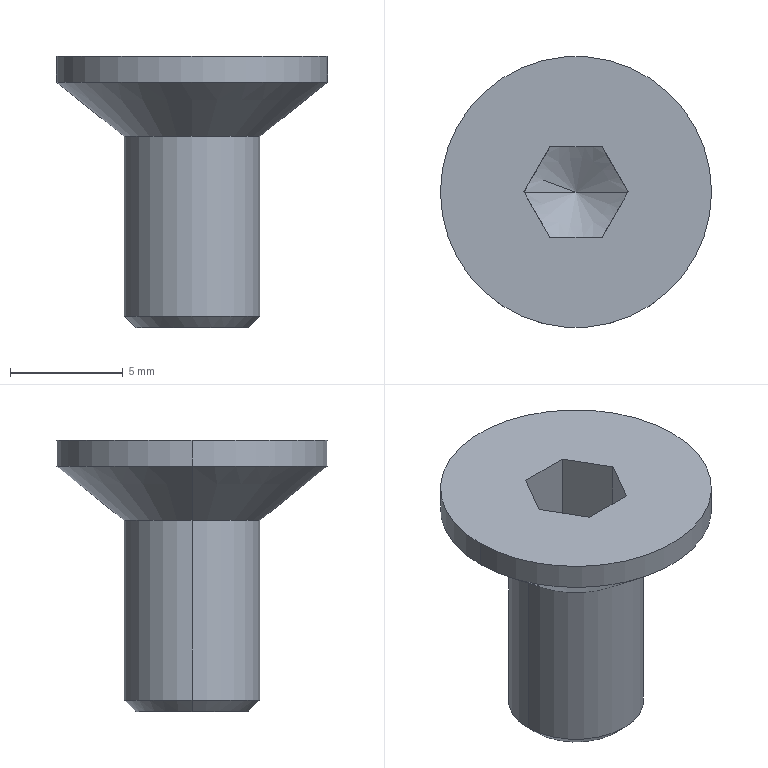Part | Creo | 1 solid | 18 faces | box 12 x 12 x 12 mm | volume 475.431 mm3 | plane 8 | cone 6 | cylinder 4 | commonest cylinder face diameters 6 x2 12 x2
STEP:
#1=CARTESIAN_POINT('',(219.809,61.745,-57.491));
#2=VERTEX_POINT('',#1);
#3=CARTESIAN_POINT('',(218.655,63.745,-57.491));
#4=VERTEX_POINT('',#3);
#5=CARTESIAN_POINT('',(219.809,61.745,-57.491));
#6=CARTESIAN_POINT('',(219.756,61.838,-57.522));
#7=CARTESIAN_POINT('',(219.648,62.026,-57.578));
#8=CARTESIAN_POINT('',(219.482,62.312,-57.639));
#9=CARTESIAN_POINT('',(219.315,62.601,-57.671));
#10=CARTESIAN_POINT('',(219.148,62.891,-57.671));
#11=CARTESIAN_POINT('',(218.981,63.18,-57.639));
#12=CARTESIAN_POINT('',(218.816,63.466,-57.578));
#13=CARTESIAN_POINT('',(218.708,63.653,-57.522));
#14=CARTESIAN_POINT('',(218.655,63.745,-57.491));
#15=B_SPLINE_CURVE_WITH_KNOTS('',3,(#5,#6,#7,#8,#9,#10,#11,#12,#13,#14),.UNSPECIFIED.,.F.,.F.,(4,1,1,1,1,1,1,4),(0.,0.1429,0.2857,0.4286,0.5714,0.7143,0.8571,1.),.UNSPECIFIED.);
#16=EDGE_CURVE('',#2,#4,#15,.T.);
#17=ORIENTED_EDGE('',*,*,#16,.F.);
#18=CARTESIAN_POINT('',(217.5,61.745,-58.824));
#19=VERTEX_POINT('',#18);
#20=CARTESIAN_POINT('',(217.5,61.745,-58.824));
#21=DIRECTION('',(0.866,0.,0.5));
#22=VECTOR('',#21,2.667);
#23=LINE('',#20,#22);
#24=EDGE_CURVE('',#19,#2,#23,.T.);
#25=ORIENTED_EDGE('',*,*,#24,.F.);
#26=CARTESIAN_POINT('',(215.191,61.745,-57.491));
#27=VERTEX_POINT('',#26);
#28=CARTESIAN_POINT('',(217.5,61.745,-58.824));
#29=DIRECTION('',(-0.866,0.,0.5));
#30=VECTOR('',#29,2.667);
#31=LINE('',#28,#30);
#32=EDGE_CURVE('',#19,#27,#31,.T.);
#33=ORIENTED_EDGE('',*,*,#32,.T.);
#34=CARTESIAN_POINT('',(216.345,63.745,-57.491));
#35=VERTEX_POINT('',#34);
#36=CARTESIAN_POINT('',(216.345,63.745,-57.491));
#37=CARTESIAN_POINT('',(216.292,63.653,-57.522));
#38=CARTESIAN_POINT('',(216.184,63.466,-57.578));
#39=CARTESIAN_POINT('',(216.019,63.18,-57.639));
#40=CARTESIAN_POINT('',(215.852,62.891,-57.671));
#41=CARTESIAN_POINT('',(215.685,62.601,-57.671));
#42=CARTESIAN_POINT('',(215.518,62.312,-57.639));
#43=CARTESIAN_POINT('',(215.352,62.026,-57.578));
#44=CARTESIAN_POINT('',(215.244,61.838,-57.522));
#45=CARTESIAN_POINT('',(215.191,61.745,-57.491));
#46=B_SPLINE_CURVE_WITH_KNOTS('',3,(#36,#37,#38,#39,#40,#41,#42,#43,#44,#45),.UNSPECIFIED.,.F.,.F.,(4,1,1,1,1,1,1,4),(0.,0.1429,0.2857,0.4286,0.5714,0.7143,0.8571,1.),.UNSPECIFIED.);
#47=EDGE_CURVE('',#35,#27,#46,.T.);
#48=ORIENTED_EDGE('',*,*,#47,.F.);
#49=CARTESIAN_POINT('',(218.655,63.745,-57.491));
#50=CARTESIAN_POINT('',(218.597,63.745,-57.508));
#51=CARTESIAN_POINT('',(218.483,63.745,-57.539));
#52=CARTESIAN_POINT('',(218.318,63.745,-57.578));
#53=CARTESIAN_POINT('',(218.156,63.745,-57.61));
#54=CARTESIAN_POINT('',(217.994,63.745,-57.636));
#55=CARTESIAN_POINT('',(217.831,63.745,-57.655));
#56=CARTESIAN_POINT('',(217.666,63.745,-57.667));
#57=CARTESIAN_POINT('',(217.5,63.745,-57.671));
#58=CARTESIAN_POINT('',(217.334,63.745,-57.667));
#59=CARTESIAN_POINT('',(217.169,63.745,-57.655));
#60=CARTESIAN_POINT('',(217.006,63.745,-57.636));
#61=CARTESIAN_POINT('',(216.844,63.745,-57.61));
#62=CARTESIAN_POINT('',(216.682,63.745,-57.578));
#63=CARTESIAN_POINT('',(216.517,63.745,-57.539));
#64=CARTESIAN_POINT('',(216.403,63.745,-57.508));
#65=CARTESIAN_POINT('',(216.345,63.745,-57.491));
#66=B_SPLINE_CURVE_WITH_KNOTS('',3,(#49,#50,#51,#52,#53,#54,#55,#56,#57,#58,#59,#60,#61,#62,#63,#64,#65),.UNSPECIFIED.,.F.,.F.,(4,1,1,1,1,1,1,1,1,1,1,1,1,1,4),(0.,0.07143,0.1429,0.2143,0.2857,0.3571,0.4286,0.5,0.5714,0.6429,0.7143,0.7857,0.8571,0.9286,1.),.UNSPECIFIED.);
#67=EDGE_CURVE('',#4,#35,#66,.T.);
#68=ORIENTED_EDGE('',*,*,#67,.F.);
#69=EDGE_LOOP('',(#17,#25,#33,#48,#68));
#70=FACE_OUTER_BOUND('',#69,.F.);
#71=CARTESIAN_POINT('',(217.5,61.745,-58.144));
#72=DIRECTION('',(0.,0.,1.));
#73=DIRECTION('',(1.,0.,0.));
#74=AXIS2_PLACEMENT_3D('',#71,#72,#73);
#75=CONICAL_SURFACE('',#74,1.178,60.);
#76=ADVANCED_FACE('',(#70),#75,.F.);
#77=CARTESIAN_POINT('',(218.655,63.745,-54.491));
#78=VERTEX_POINT('',#77);
#79=CARTESIAN_POINT('',(219.809,61.745,-54.491));
#80=VERTEX_POINT('',#79);
#81=CARTESIAN_POINT('',(218.655,63.745,-54.491));
#82=DIRECTION('',(0.5,-0.866,0.));
#83=VECTOR('',#82,2.309);
#84=LINE('',#81,#83);
#85=EDGE_CURVE('',#78,#80,#84,.T.);
#86=ORIENTED_EDGE('',*,*,#85,.T.);
#87=CARTESIAN_POINT('',(219.809,61.745,-54.491));
#88=DIRECTION('',(0.,0.,-1.));
#89=VECTOR('',#88,3.);
#90=LINE('',#87,#89);
#91=EDGE_CURVE('',#80,#2,#90,.T.);
#92=ORIENTED_EDGE('',*,*,#91,.T.);
#93=ORIENTED_EDGE('',*,*,#16,.T.);
#94=CARTESIAN_POINT('',(218.655,63.745,-54.491));
#95=DIRECTION('',(0.,0.,-1.));
#96=VECTOR('',#95,3.);
#97=LINE('',#94,#96);
#98=EDGE_CURVE('',#78,#4,#97,.T.);
#99=ORIENTED_EDGE('',*,*,#98,.F.);
#100=EDGE_LOOP('',(#86,#92,#93,#99));
#101=FACE_OUTER_BOUND('',#100,.F.);
#102=CARTESIAN_POINT('',(219.809,61.745,-57.491));
#103=DIRECTION('',(0.866,0.5,0.));
#104=DIRECTION('',(-0.5,0.866,0.));
#105=AXIS2_PLACEMENT_3D('',#102,#103,#104);
#106=PLANE('',#105);
#107=ADVANCED_FACE('',(#101),#106,.F.);
#108=CARTESIAN_POINT('',(223.5,61.745,-54.491));
#109=VERTEX_POINT('',#108);
#110=CARTESIAN_POINT('',(211.5,61.745,-54.491));
#111=VERTEX_POINT('',#110);
#112=CARTESIAN_POINT('',(217.5,61.745,-54.491));
#113=DIRECTION('',(0.,0.,1.));
#114=DIRECTION('',(1.,0.,0.));
#115=AXIS2_PLACEMENT_3D('',#112,#113,#114);
#116=CIRCLE('',#115,6.);
#117=EDGE_CURVE('',#109,#111,#116,.T.);
#118=ORIENTED_EDGE('',*,*,#117,.F.);
#119=CARTESIAN_POINT('',(217.5,61.745,-54.491));
#120=DIRECTION('',(0.,0.,1.));
#121=DIRECTION('',(-1.,0.,0.));
#122=AXIS2_PLACEMENT_3D('',#119,#120,#121);
#123=CIRCLE('',#122,6.);
#124=EDGE_CURVE('',#111,#109,#123,.T.);
#125=ORIENTED_EDGE('',*,*,#124,.F.);
#126=EDGE_LOOP('',(#118,#125));
#127=FACE_OUTER_BOUND('',#126,.F.);
#128=CARTESIAN_POINT('',(216.345,63.745,-54.491));
#129=VERTEX_POINT('',#128);
#130=CARTESIAN_POINT('',(216.345,63.745,-54.491));
#131=DIRECTION('',(1.,0.,0.));
#132=VECTOR('',#131,2.309);
#133=LINE('',#130,#132);
#134=EDGE_CURVE('',#129,#78,#133,.T.);
#135=ORIENTED_EDGE('',*,*,#134,.F.);
#136=CARTESIAN_POINT('',(215.191,61.745,-54.491));
#137=VERTEX_POINT('',#136);
#138=CARTESIAN_POINT('',(215.191,61.745,-54.491));
#139=DIRECTION('',(0.5,0.866,0.));
#140=VECTOR('',#139,2.309);
#141=LINE('',#138,#140);
#142=EDGE_CURVE('',#137,#129,#141,.T.);
#143=ORIENTED_EDGE('',*,*,#142,.F.);
#144=CARTESIAN_POINT('',(216.345,59.745,-54.491));
#145=VERTEX_POINT('',#144);
#146=CARTESIAN_POINT('',(216.345,59.745,-54.491));
#147=DIRECTION('',(-0.5,0.866,0.));
#148=VECTOR('',#147,2.309);
#149=LINE('',#146,#148);
#150=EDGE_CURVE('',#145,#137,#149,.T.);
#151=ORIENTED_EDGE('',*,*,#150,.F.);
#152=CARTESIAN_POINT('',(218.655,59.745,-54.491));
#153=VERTEX_POINT('',#152);
#154=CARTESIAN_POINT('',(218.655,59.745,-54.491));
#155=DIRECTION('',(-1.,0.,0.));
#156=VECTOR('',#155,2.309);
#157=LINE('',#154,#156);
#158=EDGE_CURVE('',#153,#145,#157,.T.);
#159=ORIENTED_EDGE('',*,*,#158,.F.);
#160=CARTESIAN_POINT('',(219.809,61.745,-54.491));
#161=DIRECTION('',(-0.5,-0.866,0.));
#162=VECTOR('',#161,2.309);
#163=LINE('',#160,#162);
#164=EDGE_CURVE('',#80,#153,#163,.T.);
#165=ORIENTED_EDGE('',*,*,#164,.F.);
#166=ORIENTED_EDGE('',*,*,#85,.F.);
#167=EDGE_LOOP('',(#135,#143,#151,#159,#165,#166));
#168=FACE_BOUND('',#167,.F.);
#169=CARTESIAN_POINT('',(223.5,61.745,-54.491));
#170=DIRECTION('',(0.,0.,-1.));
#171=DIRECTION('',(-1.,0.,0.));
#172=AXIS2_PLACEMENT_3D('',#169,#170,#171);
#173=PLANE('',#172);
#174=ADVANCED_FACE('',(#127,#168),#173,.F.);
#175=ORIENTED_EDGE('',*,*,#134,.T.);
#176=ORIENTED_EDGE('',*,*,#98,.T.);
#177=ORIENTED_EDGE('',*,*,#67,.T.);
#178=CARTESIAN_POINT('',(216.345,63.745,-54.491));
#179=DIRECTION('',(0.,0.,-1.));
#180=VECTOR('',#179,3.);
#181=LINE('',#178,#180);
#182=EDGE_CURVE('',#129,#35,#181,.T.);
#183=ORIENTED_EDGE('',*,*,#182,.F.);
#184=EDGE_LOOP('',(#175,#176,#177,#183));
#185=FACE_OUTER_BOUND('',#184,.F.);
#186=CARTESIAN_POINT('',(218.655,63.745,-57.491));
#187=DIRECTION('',(0.,1.,0.));
#188=DIRECTION('',(0.,0.,1.));
#189=AXIS2_PLACEMENT_3D('',#186,#187,#188);
#190=PLANE('',#189);
#191=ADVANCED_FACE('',(#185),#190,.F.);
#192=ORIENTED_EDGE('',*,*,#142,.T.);
#193=ORIENTED_EDGE('',*,*,#182,.T.);
#194=ORIENTED_EDGE('',*,*,#47,.T.);
#195=CARTESIAN_POINT('',(215.191,61.745,-54.491));
#196=DIRECTION('',(0.,0.,-1.));
#197=VECTOR('',#196,3.);
#198=LINE('',#195,#197);
#199=EDGE_CURVE('',#137,#27,#198,.T.);
#200=ORIENTED_EDGE('',*,*,#199,.F.);
#201=EDGE_LOOP('',(#192,#193,#194,#200));
#202=FACE_OUTER_BOUND('',#201,.F.);
#203=CARTESIAN_POINT('',(216.345,63.745,-57.491));
#204=DIRECTION('',(-0.866,0.5,0.));
#205=DIRECTION('',(-0.5,-0.866,0.));
#206=AXIS2_PLACEMENT_3D('',#203,#204,#205);
#207=PLANE('',#206);
#208=ADVANCED_FACE('',(#202),#207,.F.);
#209=ORIENTED_EDGE('',*,*,#150,.T.);
#210=ORIENTED_EDGE('',*,*,#199,.T.);
#211=CARTESIAN_POINT('',(216.345,59.745,-57.491));
#212=VERTEX_POINT('',#211);
#213=CARTESIAN_POINT('',(215.191,61.745,-57.491));
#214=CARTESIAN_POINT('',(215.244,61.652,-57.522));
#215=CARTESIAN_POINT('',(215.352,61.465,-57.578));
#216=CARTESIAN_POINT('',(215.518,61.178,-57.639));
#217=CARTESIAN_POINT('',(215.685,60.889,-57.671));
#218=CARTESIAN_POINT('',(215.852,60.6,-57.671));
#219=CARTESIAN_POINT('',(216.019,60.311,-57.639));
#220=CARTESIAN_POINT('',(216.184,60.024,-57.578));
#221=CARTESIAN_POINT('',(216.292,59.838,-57.522));
#222=CARTESIAN_POINT('',(216.345,59.745,-57.491));
#223=B_SPLINE_CURVE_WITH_KNOTS('',3,(#213,#214,#215,#216,#217,#218,#219,#220,#221,#222),.UNSPECIFIED.,.F.,.F.,(4,1,1,1,1,1,1,4),(0.,0.1429,0.2857,0.4286,0.5714,0.7143,0.8571,1.),.UNSPECIFIED.);
#224=EDGE_CURVE('',#27,#212,#223,.T.);
#225=ORIENTED_EDGE('',*,*,#224,.T.);
#226=CARTESIAN_POINT('',(216.345,59.745,-54.491));
#227=DIRECTION('',(0.,0.,-1.));
#228=VECTOR('',#227,3.);
#229=LINE('',#226,#228);
#230=EDGE_CURVE('',#145,#212,#229,.T.);
#231=ORIENTED_EDGE('',*,*,#230,.F.);
#232=EDGE_LOOP('',(#209,#210,#225,#231));
#233=FACE_OUTER_BOUND('',#232,.F.);
#234=CARTESIAN_POINT('',(215.191,61.745,-57.491));
#235=DIRECTION('',(-0.866,-0.5,0.));
#236=DIRECTION('',(0.5,-0.866,0.));
#237=AXIS2_PLACEMENT_3D('',#234,#235,#236);
#238=PLANE('',#237);
#239=ADVANCED_FACE('',(#233),#238,.F.);
#240=CARTESIAN_POINT('',(218.655,59.745,-57.491));
#241=VERTEX_POINT('',#240);
#242=CARTESIAN_POINT('',(216.345,59.745,-57.491));
#243=CARTESIAN_POINT('',(216.403,59.745,-57.508));
#244=CARTESIAN_POINT('',(216.517,59.745,-57.539));
#245=CARTESIAN_POINT('',(216.682,59.745,-57.578));
#246=CARTESIAN_POINT('',(216.844,59.745,-57.61));
#247=CARTESIAN_POINT('',(217.006,59.745,-57.636));
#248=CARTESIAN_POINT('',(217.169,59.745,-57.655));
#249=CARTESIAN_POINT('',(217.334,59.745,-57.667));
#250=CARTESIAN_POINT('',(217.5,59.745,-57.671));
#251=CARTESIAN_POINT('',(217.666,59.745,-57.667));
#252=CARTESIAN_POINT('',(217.831,59.745,-57.655));
#253=CARTESIAN_POINT('',(217.994,59.745,-57.636));
#254=CARTESIAN_POINT('',(218.156,59.745,-57.61));
#255=CARTESIAN_POINT('',(218.318,59.745,-57.578));
#256=CARTESIAN_POINT('',(218.483,59.745,-57.539));
#257=CARTESIAN_POINT('',(218.597,59.745,-57.508));
#258=CARTESIAN_POINT('',(218.655,59.745,-57.491));
#259=B_SPLINE_CURVE_WITH_KNOTS('',3,(#242,#243,#244,#245,#246,#247,#248,#249,#250,#251,#252,#253,#254,#255,#256,#257,#258),.UNSPECIFIED.,.F.,.F.,(4,1,1,1,1,1,1,1,1,1,1,1,1,1,4),(0.,0.07143,0.1429,0.2143,0.2857,0.3571,0.4286,0.5,0.5714,0.6429,0.7143,0.7857,0.8571,0.9286,1.),.UNSPECIFIED.);
#260=EDGE_CURVE('',#212,#241,#259,.T.);
#261=ORIENTED_EDGE('',*,*,#260,.F.);
#262=ORIENTED_EDGE('',*,*,#224,.F.);
#263=ORIENTED_EDGE('',*,*,#32,.F.);
#264=ORIENTED_EDGE('',*,*,#24,.T.);
#265=CARTESIAN_POINT('',(218.655,59.745,-57.491));
#266=CARTESIAN_POINT('',(218.708,59.838,-57.522));
#267=CARTESIAN_POINT('',(218.816,60.024,-57.578));
#268=CARTESIAN_POINT('',(218.981,60.311,-57.639));
#269=CARTESIAN_POINT('',(219.148,60.6,-57.671));
#270=CARTESIAN_POINT('',(219.315,60.889,-57.671));
#271=CARTESIAN_POINT('',(219.482,61.178,-57.639));
#272=CARTESIAN_POINT('',(219.648,61.465,-57.578));
#273=CARTESIAN_POINT('',(219.756,61.652,-57.522));
#274=CARTESIAN_POINT('',(219.809,61.745,-57.491));
#275=B_SPLINE_CURVE_WITH_KNOTS('',3,(#265,#266,#267,#268,#269,#270,#271,#272,#273,#274),.UNSPECIFIED.,.F.,.F.,(4,1,1,1,1,1,1,4),(0.,0.1429,0.2857,0.4286,0.5714,0.7143,0.8571,1.),.UNSPECIFIED.);
#276=EDGE_CURVE('',#241,#2,#275,.T.);
#277=ORIENTED_EDGE('',*,*,#276,.F.);
#278=EDGE_LOOP('',(#261,#262,#263,#264,#277));
#279=FACE_OUTER_BOUND('',#278,.F.);
#280=CARTESIAN_POINT('',(217.5,61.745,-58.144));
#281=DIRECTION('',(0.,0.,1.));
#282=DIRECTION('',(1.,0.,0.));
#283=AXIS2_PLACEMENT_3D('',#280,#281,#282);
#284=CONICAL_SURFACE('',#283,1.178,60.);
#285=ADVANCED_FACE('',(#279),#284,.F.);
#286=ORIENTED_EDGE('',*,*,#158,.T.);
#287=ORIENTED_EDGE('',*,*,#230,.T.);
#288=ORIENTED_EDGE('',*,*,#260,.T.);
#289=CARTESIAN_POINT('',(218.655,59.745,-54.491));
#290=DIRECTION('',(0.,0.,-1.));
#291=VECTOR('',#290,3.);
#292=LINE('',#289,#291);
#293=EDGE_CURVE('',#153,#241,#292,.T.);
#294=ORIENTED_EDGE('',*,*,#293,.F.);
#295=EDGE_LOOP('',(#286,#287,#288,#294));
#296=FACE_OUTER_BOUND('',#295,.F.);
#297=CARTESIAN_POINT('',(216.345,59.745,-57.491));
#298=DIRECTION('',(0.,-1.,0.));
#299=DIRECTION('',(0.,0.,-1.));
#300=AXIS2_PLACEMENT_3D('',#297,#298,#299);
#301=PLANE('',#300);
#302=ADVANCED_FACE('',(#296),#301,.F.);
#303=ORIENTED_EDGE('',*,*,#164,.T.);
#304=ORIENTED_EDGE('',*,*,#293,.T.);
#305=ORIENTED_EDGE('',*,*,#276,.T.);
#306=ORIENTED_EDGE('',*,*,#91,.F.);
#307=EDGE_LOOP('',(#303,#304,#305,#306));
#308=FACE_OUTER_BOUND('',#307,.F.);
#309=CARTESIAN_POINT('',(218.655,59.745,-57.491));
#310=DIRECTION('',(0.866,-0.5,0.));
#311=DIRECTION('',(0.5,0.866,0.));
#312=AXIS2_PLACEMENT_3D('',#309,#310,#311);
#313=PLANE('',#312);
#314=ADVANCED_FACE('',(#308),#313,.F.);
#315=ORIENTED_EDGE('',*,*,#117,.T.);
#316=CARTESIAN_POINT('',(211.5,61.745,-55.631));
#317=VERTEX_POINT('',#316);
#318=CARTESIAN_POINT('',(211.5,61.745,-55.631));
#319=DIRECTION('',(0.,0.,1.));
#320=VECTOR('',#319,1.14);
#321=LINE('',#318,#320);
#322=EDGE_CURVE('',#317,#111,#321,.T.);
#323=ORIENTED_EDGE('',*,*,#322,.F.);
#324=CARTESIAN_POINT('',(223.5,61.745,-55.631));
#325=VERTEX_POINT('',#324);
#326=CARTESIAN_POINT('',(217.5,61.745,-55.631));
#327=DIRECTION('',(0.,0.,-1.));
#328=DIRECTION('',(-1.,0.,0.));
#329=AXIS2_PLACEMENT_3D('',#326,#327,#328);
#330=CIRCLE('',#329,6.);
#331=EDGE_CURVE('',#317,#325,#330,.T.);
#332=ORIENTED_EDGE('',*,*,#331,.T.);
#333=CARTESIAN_POINT('',(223.5,61.745,-55.631));
#334=DIRECTION('',(0.,0.,1.));
#335=VECTOR('',#334,1.14);
#336=LINE('',#333,#335);
#337=EDGE_CURVE('',#325,#109,#336,.T.);
#338=ORIENTED_EDGE('',*,*,#337,.T.);
#339=EDGE_LOOP('',(#315,#323,#332,#338));
#340=FACE_OUTER_BOUND('',#339,.F.);
#341=CARTESIAN_POINT('',(217.5,61.745,-53.491));
#342=DIRECTION('',(0.,0.,1.));
#343=DIRECTION('',(1.,0.,0.));
#344=AXIS2_PLACEMENT_3D('',#341,#342,#343);
#345=CYLINDRICAL_SURFACE('',#344,6.);
#346=ADVANCED_FACE('',(#340),#345,.T.);
#347=ORIENTED_EDGE('',*,*,#124,.T.);
#348=ORIENTED_EDGE('',*,*,#337,.F.);
#349=CARTESIAN_POINT('',(217.5,61.745,-55.631));
#350=DIRECTION('',(0.,0.,-1.));
#351=DIRECTION('',(1.,0.,0.));
#352=AXIS2_PLACEMENT_3D('',#349,#350,#351);
#353=CIRCLE('',#352,6.);
#354=EDGE_CURVE('',#325,#317,#353,.T.);
#355=ORIENTED_EDGE('',*,*,#354,.T.);
#356=ORIENTED_EDGE('',*,*,#322,.T.);
#357=EDGE_LOOP('',(#347,#348,#355,#356));
#358=FACE_OUTER_BOUND('',#357,.F.);
#359=CARTESIAN_POINT('',(217.5,61.745,-53.491));
#360=DIRECTION('',(0.,0.,1.));
#361=DIRECTION('',(1.,0.,0.));
#362=AXIS2_PLACEMENT_3D('',#359,#360,#361);
#363=CYLINDRICAL_SURFACE('',#362,6.);
#364=ADVANCED_FACE('',(#358),#363,.T.);
#365=CARTESIAN_POINT('',(214.5,61.745,-58.031));
#366=VERTEX_POINT('',#365);
#367=CARTESIAN_POINT('',(220.5,61.745,-58.031));
#368=VERTEX_POINT('',#367);
#369=CARTESIAN_POINT('',(217.5,61.745,-58.031));
#370=DIRECTION('',(0.,0.,1.));
#371=DIRECTION('',(-1.,0.,0.));
#372=AXIS2_PLACEMENT_3D('',#369,#370,#371);
#373=CIRCLE('',#372,3.);
#374=EDGE_CURVE('',#366,#368,#373,.T.);
#375=ORIENTED_EDGE('',*,*,#374,.F.);
#376=CARTESIAN_POINT('',(214.5,61.745,-58.031));
#377=DIRECTION('',(-0.7809,0.,0.6247));
#378=VECTOR('',#377,3.842);
#379=LINE('',#376,#378);
#380=EDGE_CURVE('',#366,#317,#379,.T.);
#381=ORIENTED_EDGE('',*,*,#380,.T.);
#382=ORIENTED_EDGE('',*,*,#354,.F.);
#383=CARTESIAN_POINT('',(220.5,61.745,-58.031));
#384=DIRECTION('',(0.7809,0.,0.6247));
#385=VECTOR('',#384,3.842);
#386=LINE('',#383,#385);
#387=EDGE_CURVE('',#368,#325,#386,.T.);
#388=ORIENTED_EDGE('',*,*,#387,.F.);
#389=EDGE_LOOP('',(#375,#381,#382,#388));
#390=FACE_OUTER_BOUND('',#389,.F.);
#391=CARTESIAN_POINT('',(217.5,61.745,-56.831));
#392=DIRECTION('',(0.,0.,1.));
#393=DIRECTION('',(1.,0.,0.));
#394=AXIS2_PLACEMENT_3D('',#391,#392,#393);
#395=CONICAL_SURFACE('',#394,4.5,51.34);
#396=ADVANCED_FACE('',(#390),#395,.T.);
#397=ORIENTED_EDGE('',*,*,#374,.T.);
#398=CARTESIAN_POINT('',(220.5,61.745,-65.991));
#399=VERTEX_POINT('',#398);
#400=CARTESIAN_POINT('',(220.5,61.745,-65.991));
#401=DIRECTION('',(0.,0.,1.));
#402=VECTOR('',#401,7.96);
#403=LINE('',#400,#402);
#404=EDGE_CURVE('',#399,#368,#403,.T.);
#405=ORIENTED_EDGE('',*,*,#404,.F.);
#406=CARTESIAN_POINT('',(214.5,61.745,-65.991));
#407=VERTEX_POINT('',#406);
#408=CARTESIAN_POINT('',(217.5,61.745,-65.991));
#409=DIRECTION('',(0.,0.,-1.));
#410=DIRECTION('',(1.,0.,0.));
#411=AXIS2_PLACEMENT_3D('',#408,#409,#410);
#412=CIRCLE('',#411,3.);
#413=EDGE_CURVE('',#399,#407,#412,.T.);
#414=ORIENTED_EDGE('',*,*,#413,.T.);
#415=CARTESIAN_POINT('',(214.5,61.745,-65.991));
#416=DIRECTION('',(0.,0.,1.));
#417=VECTOR('',#416,7.96);
#418=LINE('',#415,#417);
#419=EDGE_CURVE('',#407,#366,#418,.T.);
#420=ORIENTED_EDGE('',*,*,#419,.T.);
#421=EDGE_LOOP('',(#397,#405,#414,#420));
#422=FACE_OUTER_BOUND('',#421,.F.);
#423=CARTESIAN_POINT('',(217.5,61.745,-53.491));
#424=DIRECTION('',(0.,0.,1.));
#425=DIRECTION('',(1.,0.,0.));
#426=AXIS2_PLACEMENT_3D('',#423,#424,#425);
#427=CYLINDRICAL_SURFACE('',#426,3.);
#428=ADVANCED_FACE('',(#422),#427,.T.);
#429=CARTESIAN_POINT('',(217.5,61.745,-58.031));
#430=DIRECTION('',(0.,0.,1.));
#431=DIRECTION('',(1.,0.,0.));
#432=AXIS2_PLACEMENT_3D('',#429,#430,#431);
#433=CIRCLE('',#432,3.);
#434=EDGE_CURVE('',#368,#366,#433,.T.);
#435=ORIENTED_EDGE('',*,*,#434,.T.);
#436=ORIENTED_EDGE('',*,*,#419,.F.);
#437=CARTESIAN_POINT('',(217.5,61.745,-65.991));
#438=DIRECTION('',(0.,0.,-1.));
#439=DIRECTION('',(-1.,0.,0.));
#440=AXIS2_PLACEMENT_3D('',#437,#438,#439);
#441=CIRCLE('',#440,3.);
#442=EDGE_CURVE('',#407,#399,#441,.T.);
#443=ORIENTED_EDGE('',*,*,#442,.T.);
#444=ORIENTED_EDGE('',*,*,#404,.T.);
#445=EDGE_LOOP('',(#435,#436,#443,#444));
#446=FACE_OUTER_BOUND('',#445,.F.);
#447=CARTESIAN_POINT('',(217.5,61.745,-53.491));
#448=DIRECTION('',(0.,0.,1.));
#449=DIRECTION('',(1.,0.,0.));
#450=AXIS2_PLACEMENT_3D('',#447,#448,#449);
#451=CYLINDRICAL_SURFACE('',#450,3.);
#452=ADVANCED_FACE('',(#446),#451,.T.);
#453=ORIENTED_EDGE('',*,*,#434,.F.);
#454=ORIENTED_EDGE('',*,*,#387,.T.);
#455=ORIENTED_EDGE('',*,*,#331,.F.);
#456=ORIENTED_EDGE('',*,*,#380,.F.);
#457=EDGE_LOOP('',(#453,#454,#455,#456));
#458=FACE_OUTER_BOUND('',#457,.F.);
#459=CARTESIAN_POINT('',(217.5,61.745,-56.831));
#460=DIRECTION('',(0.,0.,1.));
#461=DIRECTION('',(1.,0.,0.));
#462=AXIS2_PLACEMENT_3D('',#459,#460,#461);
#463=CONICAL_SURFACE('',#462,4.5,51.34);
#464=ADVANCED_FACE('',(#458),#463,.T.);
#465=ORIENTED_EDGE('',*,*,#442,.F.);
#466=CARTESIAN_POINT('',(215.,61.745,-66.491));
#467=VERTEX_POINT('',#466);
#468=CARTESIAN_POINT('',(215.,61.745,-66.491));
#469=DIRECTION('',(-0.7071,0.,0.7071));
#470=VECTOR('',#469,0.7071);
#471=LINE('',#468,#470);
#472=EDGE_CURVE('',#467,#407,#471,.T.);
#473=ORIENTED_EDGE('',*,*,#472,.F.);
#474=CARTESIAN_POINT('',(220.,61.745,-66.491));
#475=VERTEX_POINT('',#474);
#476=CARTESIAN_POINT('',(217.5,61.745,-66.491));
#477=DIRECTION('',(0.,0.,-1.));
#478=DIRECTION('',(-1.,0.,0.));
#479=AXIS2_PLACEMENT_3D('',#476,#477,#478);
#480=CIRCLE('',#479,2.5);
#481=EDGE_CURVE('',#467,#475,#480,.T.);
#482=ORIENTED_EDGE('',*,*,#481,.T.);
#483=CARTESIAN_POINT('',(220.,61.745,-66.491));
#484=DIRECTION('',(0.7071,0.,0.7071));
#485=VECTOR('',#484,0.7071);
#486=LINE('',#483,#485);
#487=EDGE_CURVE('',#475,#399,#486,.T.);
#488=ORIENTED_EDGE('',*,*,#487,.T.);
#489=EDGE_LOOP('',(#465,#473,#482,#488));
#490=FACE_OUTER_BOUND('',#489,.F.);
#491=CARTESIAN_POINT('',(217.5,61.745,-66.241));
#492=DIRECTION('',(0.,0.,1.));
#493=DIRECTION('',(1.,0.,0.));
#494=AXIS2_PLACEMENT_3D('',#491,#492,#493);
#495=CONICAL_SURFACE('',#494,2.75,45.);
#496=ADVANCED_FACE('',(#490),#495,.T.);
#497=ORIENTED_EDGE('',*,*,#413,.F.);
#498=ORIENTED_EDGE('',*,*,#487,.F.);
#499=CARTESIAN_POINT('',(217.5,61.745,-66.491));
#500=DIRECTION('',(0.,0.,-1.));
#501=DIRECTION('',(1.,0.,0.));
#502=AXIS2_PLACEMENT_3D('',#499,#500,#501);
#503=CIRCLE('',#502,2.5);
#504=EDGE_CURVE('',#475,#467,#503,.T.);
#505=ORIENTED_EDGE('',*,*,#504,.T.);
#506=ORIENTED_EDGE('',*,*,#472,.T.);
#507=EDGE_LOOP('',(#497,#498,#505,#506));
#508=FACE_OUTER_BOUND('',#507,.F.);
#509=CARTESIAN_POINT('',(217.5,61.745,-66.241));
#510=DIRECTION('',(0.,0.,1.));
#511=DIRECTION('',(1.,0.,0.));
#512=AXIS2_PLACEMENT_3D('',#509,#510,#511);
#513=CONICAL_SURFACE('',#512,2.75,45.);
#514=ADVANCED_FACE('',(#508),#513,.T.);
#515=ORIENTED_EDGE('',*,*,#504,.F.);
#516=ORIENTED_EDGE('',*,*,#481,.F.);
#517=EDGE_LOOP('',(#515,#516));
#518=FACE_OUTER_BOUND('',#517,.F.);
#519=CARTESIAN_POINT('',(217.5,61.745,-66.491));
#520=DIRECTION('',(0.,0.,1.));
#521=DIRECTION('',(1.,0.,0.));
#522=AXIS2_PLACEMENT_3D('',#519,#520,#521);
#523=PLANE('',#522);
#524=ADVANCED_FACE('',(#518),#523,.F.);
#525=CLOSED_SHELL('',(#76,#107,#174,#191,#208,#239,#285,#302,#314,#346,#364,#396,#428,#452,#464,#496,#514,#524));
#526=MANIFOLD_SOLID_BREP('',#525);
#527=(LENGTH_UNIT()NAMED_UNIT(*)SI_UNIT(.MILLI.,.METRE.));
#528=UNCERTAINTY_MEASURE_WITH_UNIT(LENGTH_MEASURE(0.002078),#527,'','');
#529=(NAMED_UNIT(*)PLANE_ANGLE_UNIT()SI_UNIT($,.RADIAN.));
#530=PLANE_ANGLE_MEASURE_WITH_UNIT(PLANE_ANGLE_MEASURE(0.01745),#529);
#531=(CONVERSION_BASED_UNIT('DEGREE',#530)NAMED_UNIT(*)PLANE_ANGLE_UNIT());
#532=(NAMED_UNIT(*)SI_UNIT($,.STERADIAN.)SOLID_ANGLE_UNIT());
#533=(GEOMETRIC_REPRESENTATION_CONTEXT(3)GLOBAL_UNCERTAINTY_ASSIGNED_CONTEXT((#528))GLOBAL_UNIT_ASSIGNED_CONTEXT((#527,#531,#532))REPRESENTATION_CONTEXT('',''));
#534=ADVANCED_BREP_SHAPE_REPRESENTATION('',(#526),#533);